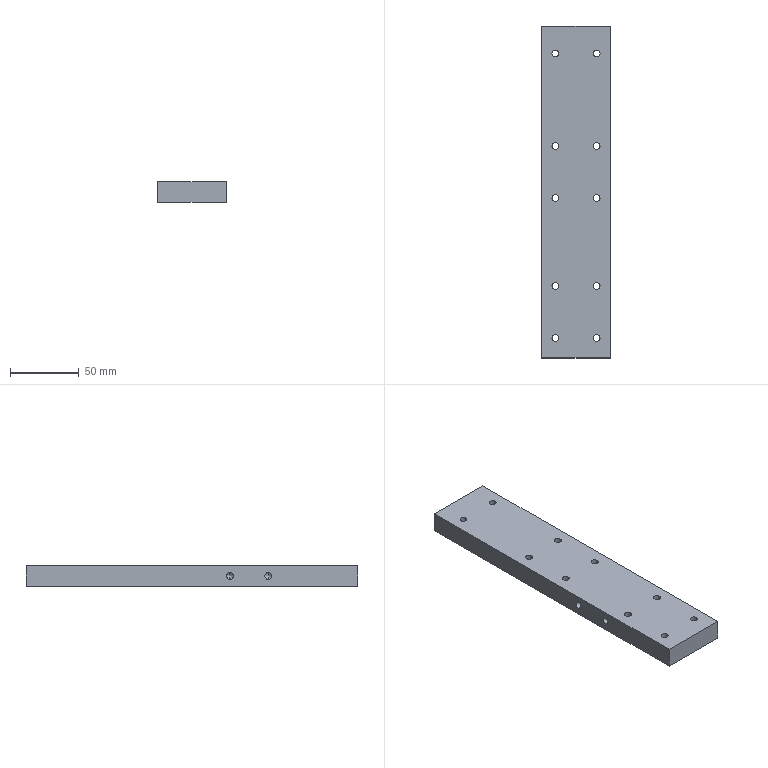Part | 1 solid | 50 faces | box 50 x 242 x 15 mm | volume 176198 mm3 | cylinder 32 | cone 12 | plane 6 | commonest cylinder face diameters 5 x28 6.8 x4
STEP:
#1=CARTESIAN_POINT('',(12.5,124.,15.));
#2=VERTEX_POINT('',#1);
#3=CARTESIAN_POINT('',(17.5,124.,15.));
#4=VERTEX_POINT('',#3);
#5=CARTESIAN_POINT('',(15.,124.,15.));
#6=DIRECTION('',(0.,0.,1.));
#7=DIRECTION('',(1.,0.,0.));
#8=AXIS2_PLACEMENT_3D('',#5,#6,#7);
#9=CIRCLE('',#8,2.5);
#10=EDGE_CURVE('',#2,#4,#9,.T.);
#11=ORIENTED_EDGE('',*,*,#10,.T.);
#12=CARTESIAN_POINT('',(17.5,124.,0.));
#13=VERTEX_POINT('',#12);
#14=CARTESIAN_POINT('',(17.5,124.,0.));
#15=DIRECTION('',(0.,0.,-1.));
#16=VECTOR('',#15,1000.);
#17=LINE('',#14,#16);
#18=EDGE_CURVE('',#4,#13,#17,.T.);
#19=ORIENTED_EDGE('',*,*,#18,.T.);
#20=CARTESIAN_POINT('',(12.5,124.,0.));
#21=VERTEX_POINT('',#20);
#22=CARTESIAN_POINT('',(15.,124.,0.));
#23=DIRECTION('',(0.,0.,-1.));
#24=DIRECTION('',(-1.,0.,0.));
#25=AXIS2_PLACEMENT_3D('',#22,#23,#24);
#26=CIRCLE('',#25,2.5);
#27=EDGE_CURVE('',#13,#21,#26,.T.);
#28=ORIENTED_EDGE('',*,*,#27,.T.);
#29=CARTESIAN_POINT('',(12.5,124.,0.));
#30=DIRECTION('',(0.,0.,-1.));
#31=VECTOR('',#30,1000.);
#32=LINE('',#29,#31);
#33=EDGE_CURVE('',#2,#21,#32,.T.);
#34=ORIENTED_EDGE('',*,*,#33,.F.);
#35=EDGE_LOOP('',(#11,#19,#28,#34));
#36=FACE_OUTER_BOUND('',#35,.T.);
#37=CARTESIAN_POINT('',(15.,124.,0.));
#38=DIRECTION('',(0.,0.,-1.));
#39=DIRECTION('',(-1.,0.,0.));
#40=AXIS2_PLACEMENT_3D('',#37,#38,#39);
#41=CYLINDRICAL_SURFACE('',#40,2.5);
#42=ADVANCED_FACE('',(#36),#41,.F.);
#43=CARTESIAN_POINT('',(-17.5,124.,15.));
#44=VERTEX_POINT('',#43);
#45=CARTESIAN_POINT('',(-12.5,124.,15.));
#46=VERTEX_POINT('',#45);
#47=CARTESIAN_POINT('',(-15.,124.,15.));
#48=DIRECTION('',(0.,0.,1.));
#49=DIRECTION('',(1.,0.,0.));
#50=AXIS2_PLACEMENT_3D('',#47,#48,#49);
#51=CIRCLE('',#50,2.5);
#52=EDGE_CURVE('',#44,#46,#51,.T.);
#53=ORIENTED_EDGE('',*,*,#52,.T.);
#54=CARTESIAN_POINT('',(-12.5,124.,0.));
#55=VERTEX_POINT('',#54);
#56=CARTESIAN_POINT('',(-12.5,124.,0.));
#57=DIRECTION('',(0.,0.,-1.));
#58=VECTOR('',#57,1000.);
#59=LINE('',#56,#58);
#60=EDGE_CURVE('',#46,#55,#59,.T.);
#61=ORIENTED_EDGE('',*,*,#60,.T.);
#62=CARTESIAN_POINT('',(-17.5,124.,0.));
#63=VERTEX_POINT('',#62);
#64=CARTESIAN_POINT('',(-15.,124.,0.));
#65=DIRECTION('',(0.,0.,-1.));
#66=DIRECTION('',(-1.,0.,0.));
#67=AXIS2_PLACEMENT_3D('',#64,#65,#66);
#68=CIRCLE('',#67,2.5);
#69=EDGE_CURVE('',#55,#63,#68,.T.);
#70=ORIENTED_EDGE('',*,*,#69,.T.);
#71=CARTESIAN_POINT('',(-17.5,124.,0.));
#72=DIRECTION('',(0.,0.,-1.));
#73=VECTOR('',#72,1000.);
#74=LINE('',#71,#73);
#75=EDGE_CURVE('',#44,#63,#74,.T.);
#76=ORIENTED_EDGE('',*,*,#75,.F.);
#77=EDGE_LOOP('',(#53,#61,#70,#76));
#78=FACE_OUTER_BOUND('',#77,.T.);
#79=CARTESIAN_POINT('',(-15.,124.,0.));
#80=DIRECTION('',(0.,0.,-1.));
#81=DIRECTION('',(-1.,0.,0.));
#82=AXIS2_PLACEMENT_3D('',#79,#80,#81);
#83=CYLINDRICAL_SURFACE('',#82,2.5);
#84=ADVANCED_FACE('',(#78),#83,.F.);
#85=CARTESIAN_POINT('',(-15.,129.,4.1));
#86=VERTEX_POINT('',#85);
#87=CARTESIAN_POINT('',(-15.,129.,10.9));
#88=VERTEX_POINT('',#87);
#89=CARTESIAN_POINT('',(-15.,129.,7.5));
#90=DIRECTION('',(0.,1.,0.));
#91=DIRECTION('',(0.,0.,1.));
#92=AXIS2_PLACEMENT_3D('',#89,#90,#91);
#93=CIRCLE('',#92,3.4);
#94=EDGE_CURVE('',#86,#88,#93,.T.);
#95=ORIENTED_EDGE('',*,*,#94,.F.);
#96=CARTESIAN_POINT('',(-15.,144.,4.1));
#97=VERTEX_POINT('',#96);
#98=CARTESIAN_POINT('',(-15.,144.,4.1));
#99=DIRECTION('',(0.,1.,0.));
#100=VECTOR('',#99,1000.);
#101=LINE('',#98,#100);
#102=EDGE_CURVE('',#86,#97,#101,.T.);
#103=ORIENTED_EDGE('',*,*,#102,.T.);
#104=CARTESIAN_POINT('',(-15.,144.,10.9));
#105=VERTEX_POINT('',#104);
#106=CARTESIAN_POINT('',(-15.,144.,7.5));
#107=DIRECTION('',(0.,1.,0.));
#108=DIRECTION('',(0.,0.,1.));
#109=AXIS2_PLACEMENT_3D('',#106,#107,#108);
#110=CIRCLE('',#109,3.4);
#111=EDGE_CURVE('',#97,#105,#110,.T.);
#112=ORIENTED_EDGE('',*,*,#111,.T.);
#113=CARTESIAN_POINT('',(-15.,144.,10.9));
#114=DIRECTION('',(0.,1.,0.));
#115=VECTOR('',#114,1000.);
#116=LINE('',#113,#115);
#117=EDGE_CURVE('',#88,#105,#116,.T.);
#118=ORIENTED_EDGE('',*,*,#117,.F.);
#119=EDGE_LOOP('',(#95,#103,#112,#118));
#120=FACE_OUTER_BOUND('',#119,.T.);
#121=CARTESIAN_POINT('',(-15.,144.,7.5));
#122=DIRECTION('',(0.,1.,0.));
#123=DIRECTION('',(0.,0.,1.));
#124=AXIS2_PLACEMENT_3D('',#121,#122,#123);
#125=CYLINDRICAL_SURFACE('',#124,3.4);
#126=ADVANCED_FACE('',(#120),#125,.F.);
#127=CARTESIAN_POINT('',(-15.,126.957,7.5));
#128=VERTEX_POINT('',#127);
#129=CARTESIAN_POINT('',(-15.,129.,10.9));
#130=DIRECTION('',(0.,0.515,0.8572));
#131=VECTOR('',#130,1000.);
#132=LINE('',#129,#131);
#133=EDGE_CURVE('',#128,#88,#132,.T.);
#134=ORIENTED_EDGE('',*,*,#133,.F.);
#135=CARTESIAN_POINT('',(-15.,129.,4.1));
#136=DIRECTION('',(0.,0.515,-0.8572));
#137=VECTOR('',#136,1000.);
#138=LINE('',#135,#137);
#139=EDGE_CURVE('',#128,#86,#138,.T.);
#140=ORIENTED_EDGE('',*,*,#139,.T.);
#141=ORIENTED_EDGE('',*,*,#94,.T.);
#142=EDGE_LOOP('',(#134,#140,#141));
#143=FACE_OUTER_BOUND('',#142,.T.);
#144=CARTESIAN_POINT('',(-15.,129.,7.5));
#145=DIRECTION('',(0.,1.,0.));
#146=DIRECTION('',(0.,0.,1.));
#147=AXIS2_PLACEMENT_3D('',#144,#145,#146);
#148=CONICAL_SURFACE('',#147,3.4,1.03);
#149=ADVANCED_FACE('',(#143),#148,.F.);
#150=CARTESIAN_POINT('',(15.,129.,4.1));
#151=VERTEX_POINT('',#150);
#152=CARTESIAN_POINT('',(15.,129.,10.9));
#153=VERTEX_POINT('',#152);
#154=CARTESIAN_POINT('',(15.,129.,7.5));
#155=DIRECTION('',(0.,1.,0.));
#156=DIRECTION('',(0.,0.,1.));
#157=AXIS2_PLACEMENT_3D('',#154,#155,#156);
#158=CIRCLE('',#157,3.4);
#159=EDGE_CURVE('',#151,#153,#158,.T.);
#160=ORIENTED_EDGE('',*,*,#159,.F.);
#161=CARTESIAN_POINT('',(15.,144.,4.1));
#162=VERTEX_POINT('',#161);
#163=CARTESIAN_POINT('',(15.,144.,4.1));
#164=DIRECTION('',(0.,1.,0.));
#165=VECTOR('',#164,1000.);
#166=LINE('',#163,#165);
#167=EDGE_CURVE('',#151,#162,#166,.T.);
#168=ORIENTED_EDGE('',*,*,#167,.T.);
#169=CARTESIAN_POINT('',(15.,144.,10.9));
#170=VERTEX_POINT('',#169);
#171=CARTESIAN_POINT('',(15.,144.,7.5));
#172=DIRECTION('',(0.,1.,0.));
#173=DIRECTION('',(0.,0.,1.));
#174=AXIS2_PLACEMENT_3D('',#171,#172,#173);
#175=CIRCLE('',#174,3.4);
#176=EDGE_CURVE('',#162,#170,#175,.T.);
#177=ORIENTED_EDGE('',*,*,#176,.T.);
#178=CARTESIAN_POINT('',(15.,144.,10.9));
#179=DIRECTION('',(0.,1.,0.));
#180=VECTOR('',#179,1000.);
#181=LINE('',#178,#180);
#182=EDGE_CURVE('',#153,#170,#181,.T.);
#183=ORIENTED_EDGE('',*,*,#182,.F.);
#184=EDGE_LOOP('',(#160,#168,#177,#183));
#185=FACE_OUTER_BOUND('',#184,.T.);
#186=CARTESIAN_POINT('',(15.,144.,7.5));
#187=DIRECTION('',(0.,1.,0.));
#188=DIRECTION('',(0.,0.,1.));
#189=AXIS2_PLACEMENT_3D('',#186,#187,#188);
#190=CYLINDRICAL_SURFACE('',#189,3.4);
#191=ADVANCED_FACE('',(#185),#190,.F.);
#192=CARTESIAN_POINT('',(15.,126.957,7.5));
#193=VERTEX_POINT('',#192);
#194=CARTESIAN_POINT('',(15.,129.,10.9));
#195=DIRECTION('',(0.,0.515,0.8572));
#196=VECTOR('',#195,1000.);
#197=LINE('',#194,#196);
#198=EDGE_CURVE('',#193,#153,#197,.T.);
#199=ORIENTED_EDGE('',*,*,#198,.F.);
#200=CARTESIAN_POINT('',(15.,129.,4.1));
#201=DIRECTION('',(0.,0.515,-0.8572));
#202=VECTOR('',#201,1000.);
#203=LINE('',#200,#202);
#204=EDGE_CURVE('',#193,#151,#203,.T.);
#205=ORIENTED_EDGE('',*,*,#204,.T.);
#206=ORIENTED_EDGE('',*,*,#159,.T.);
#207=EDGE_LOOP('',(#199,#205,#206));
#208=FACE_OUTER_BOUND('',#207,.T.);
#209=CARTESIAN_POINT('',(15.,129.,7.5));
#210=DIRECTION('',(0.,1.,0.));
#211=DIRECTION('',(0.,0.,1.));
#212=AXIS2_PLACEMENT_3D('',#209,#210,#211);
#213=CONICAL_SURFACE('',#212,3.4,1.03);
#214=ADVANCED_FACE('',(#208),#213,.F.);
#215=CARTESIAN_POINT('',(-10.,-4.64,5.));
#216=VERTEX_POINT('',#215);
#217=CARTESIAN_POINT('',(-10.,-4.64,10.));
#218=VERTEX_POINT('',#217);
#219=CARTESIAN_POINT('',(-10.,-4.64,7.5));
#220=DIRECTION('',(-1.,0.,0.));
#221=DIRECTION('',(0.,0.,1.));
#222=AXIS2_PLACEMENT_3D('',#219,#220,#221);
#223=CIRCLE('',#222,2.5);
#224=EDGE_CURVE('',#216,#218,#223,.T.);
#225=ORIENTED_EDGE('',*,*,#224,.F.);
#226=CARTESIAN_POINT('',(-25.,-4.64,5.));
#227=VERTEX_POINT('',#226);
#228=CARTESIAN_POINT('',(-25.,-4.64,5.));
#229=DIRECTION('',(-1.,0.,0.));
#230=VECTOR('',#229,1000.);
#231=LINE('',#228,#230);
#232=EDGE_CURVE('',#216,#227,#231,.T.);
#233=ORIENTED_EDGE('',*,*,#232,.T.);
#234=CARTESIAN_POINT('',(-25.,-4.64,10.));
#235=VERTEX_POINT('',#234);
#236=CARTESIAN_POINT('',(-25.,-4.64,7.5));
#237=DIRECTION('',(-1.,0.,0.));
#238=DIRECTION('',(0.,0.,1.));
#239=AXIS2_PLACEMENT_3D('',#236,#237,#238);
#240=CIRCLE('',#239,2.5);
#241=EDGE_CURVE('',#227,#235,#240,.T.);
#242=ORIENTED_EDGE('',*,*,#241,.T.);
#243=CARTESIAN_POINT('',(-25.,-4.64,10.));
#244=DIRECTION('',(-1.,0.,0.));
#245=VECTOR('',#244,1000.);
#246=LINE('',#243,#245);
#247=EDGE_CURVE('',#218,#235,#246,.T.);
#248=ORIENTED_EDGE('',*,*,#247,.F.);
#249=EDGE_LOOP('',(#225,#233,#242,#248));
#250=FACE_OUTER_BOUND('',#249,.T.);
#251=CARTESIAN_POINT('',(-25.,-4.64,7.5));
#252=DIRECTION('',(-1.,0.,0.));
#253=DIRECTION('',(0.,0.,1.));
#254=AXIS2_PLACEMENT_3D('',#251,#252,#253);
#255=CYLINDRICAL_SURFACE('',#254,2.5);
#256=ADVANCED_FACE('',(#250),#255,.F.);
#257=CARTESIAN_POINT('',(-8.498,-4.64,7.5));
#258=VERTEX_POINT('',#257);
#259=CARTESIAN_POINT('',(-10.,-4.64,10.));
#260=DIRECTION('',(-0.515,0.,0.8572));
#261=VECTOR('',#260,1000.);
#262=LINE('',#259,#261);
#263=EDGE_CURVE('',#258,#218,#262,.T.);
#264=ORIENTED_EDGE('',*,*,#263,.F.);
#265=CARTESIAN_POINT('',(-10.,-4.64,5.));
#266=DIRECTION('',(-0.515,0.,-0.8572));
#267=VECTOR('',#266,1000.);
#268=LINE('',#265,#267);
#269=EDGE_CURVE('',#258,#216,#268,.T.);
#270=ORIENTED_EDGE('',*,*,#269,.T.);
#271=ORIENTED_EDGE('',*,*,#224,.T.);
#272=EDGE_LOOP('',(#264,#270,#271));
#273=FACE_OUTER_BOUND('',#272,.T.);
#274=CARTESIAN_POINT('',(-10.,-4.64,7.5));
#275=DIRECTION('',(-1.,0.,0.));
#276=DIRECTION('',(0.,0.,1.));
#277=AXIS2_PLACEMENT_3D('',#274,#275,#276);
#278=CONICAL_SURFACE('',#277,2.5,1.03);
#279=ADVANCED_FACE('',(#273),#278,.F.);
#280=CARTESIAN_POINT('',(-10.,-32.64,5.));
#281=VERTEX_POINT('',#280);
#282=CARTESIAN_POINT('',(-10.,-32.64,10.));
#283=VERTEX_POINT('',#282);
#284=CARTESIAN_POINT('',(-10.,-32.64,7.5));
#285=DIRECTION('',(-1.,0.,0.));
#286=DIRECTION('',(0.,0.,1.));
#287=AXIS2_PLACEMENT_3D('',#284,#285,#286);
#288=CIRCLE('',#287,2.5);
#289=EDGE_CURVE('',#281,#283,#288,.T.);
#290=ORIENTED_EDGE('',*,*,#289,.F.);
#291=CARTESIAN_POINT('',(-25.,-32.64,5.));
#292=VERTEX_POINT('',#291);
#293=CARTESIAN_POINT('',(-25.,-32.64,5.));
#294=DIRECTION('',(-1.,0.,0.));
#295=VECTOR('',#294,1000.);
#296=LINE('',#293,#295);
#297=EDGE_CURVE('',#281,#292,#296,.T.);
#298=ORIENTED_EDGE('',*,*,#297,.T.);
#299=CARTESIAN_POINT('',(-25.,-32.64,10.));
#300=VERTEX_POINT('',#299);
#301=CARTESIAN_POINT('',(-25.,-32.64,7.5));
#302=DIRECTION('',(-1.,0.,0.));
#303=DIRECTION('',(0.,0.,1.));
#304=AXIS2_PLACEMENT_3D('',#301,#302,#303);
#305=CIRCLE('',#304,2.5);
#306=EDGE_CURVE('',#292,#300,#305,.T.);
#307=ORIENTED_EDGE('',*,*,#306,.T.);
#308=CARTESIAN_POINT('',(-25.,-32.64,10.));
#309=DIRECTION('',(-1.,0.,0.));
#310=VECTOR('',#309,1000.);
#311=LINE('',#308,#310);
#312=EDGE_CURVE('',#283,#300,#311,.T.);
#313=ORIENTED_EDGE('',*,*,#312,.F.);
#314=EDGE_LOOP('',(#290,#298,#307,#313));
#315=FACE_OUTER_BOUND('',#314,.T.);
#316=CARTESIAN_POINT('',(-25.,-32.64,7.5));
#317=DIRECTION('',(-1.,0.,0.));
#318=DIRECTION('',(0.,0.,1.));
#319=AXIS2_PLACEMENT_3D('',#316,#317,#318);
#320=CYLINDRICAL_SURFACE('',#319,2.5);
#321=ADVANCED_FACE('',(#315),#320,.F.);
#322=CARTESIAN_POINT('',(-8.498,-32.64,7.5));
#323=VERTEX_POINT('',#322);
#324=CARTESIAN_POINT('',(-10.,-32.64,10.));
#325=DIRECTION('',(-0.515,0.,0.8572));
#326=VECTOR('',#325,1000.);
#327=LINE('',#324,#326);
#328=EDGE_CURVE('',#323,#283,#327,.T.);
#329=ORIENTED_EDGE('',*,*,#328,.F.);
#330=CARTESIAN_POINT('',(-10.,-32.64,5.));
#331=DIRECTION('',(-0.515,0.,-0.8572));
#332=VECTOR('',#331,1000.);
#333=LINE('',#330,#332);
#334=EDGE_CURVE('',#323,#281,#333,.T.);
#335=ORIENTED_EDGE('',*,*,#334,.T.);
#336=ORIENTED_EDGE('',*,*,#289,.T.);
#337=EDGE_LOOP('',(#329,#335,#336));
#338=FACE_OUTER_BOUND('',#337,.T.);
#339=CARTESIAN_POINT('',(-10.,-32.64,7.5));
#340=DIRECTION('',(-1.,0.,0.));
#341=DIRECTION('',(0.,0.,1.));
#342=AXIS2_PLACEMENT_3D('',#339,#340,#341);
#343=CONICAL_SURFACE('',#342,2.5,1.03);
#344=ADVANCED_FACE('',(#338),#343,.F.);
#345=CARTESIAN_POINT('',(10.,-4.64,10.));
#346=VERTEX_POINT('',#345);
#347=CARTESIAN_POINT('',(10.,-4.64,5.));
#348=VERTEX_POINT('',#347);
#349=CARTESIAN_POINT('',(10.,-4.64,7.5));
#350=DIRECTION('',(1.,0.,0.));
#351=DIRECTION('',(0.,0.,-1.));
#352=AXIS2_PLACEMENT_3D('',#349,#350,#351);
#353=CIRCLE('',#352,2.5);
#354=EDGE_CURVE('',#346,#348,#353,.T.);
#355=ORIENTED_EDGE('',*,*,#354,.F.);
#356=CARTESIAN_POINT('',(25.,-4.64,10.));
#357=VERTEX_POINT('',#356);
#358=CARTESIAN_POINT('',(25.,-4.64,10.));
#359=DIRECTION('',(1.,0.,0.));
#360=VECTOR('',#359,1000.);
#361=LINE('',#358,#360);
#362=EDGE_CURVE('',#346,#357,#361,.T.);
#363=ORIENTED_EDGE('',*,*,#362,.T.);
#364=CARTESIAN_POINT('',(25.,-4.64,5.));
#365=VERTEX_POINT('',#364);
#366=CARTESIAN_POINT('',(25.,-4.64,7.5));
#367=DIRECTION('',(1.,0.,0.));
#368=DIRECTION('',(0.,0.,-1.));
#369=AXIS2_PLACEMENT_3D('',#366,#367,#368);
#370=CIRCLE('',#369,2.5);
#371=EDGE_CURVE('',#357,#365,#370,.T.);
#372=ORIENTED_EDGE('',*,*,#371,.T.);
#373=CARTESIAN_POINT('',(25.,-4.64,5.));
#374=DIRECTION('',(1.,0.,0.));
#375=VECTOR('',#374,1000.);
#376=LINE('',#373,#375);
#377=EDGE_CURVE('',#348,#365,#376,.T.);
#378=ORIENTED_EDGE('',*,*,#377,.F.);
#379=EDGE_LOOP('',(#355,#363,#372,#378));
#380=FACE_OUTER_BOUND('',#379,.T.);
#381=CARTESIAN_POINT('',(25.,-4.64,7.5));
#382=DIRECTION('',(1.,0.,0.));
#383=DIRECTION('',(0.,0.,-1.));
#384=AXIS2_PLACEMENT_3D('',#381,#382,#383);
#385=CYLINDRICAL_SURFACE('',#384,2.5);
#386=ADVANCED_FACE('',(#380),#385,.F.);
#387=CARTESIAN_POINT('',(8.498,-4.64,7.5));
#388=VERTEX_POINT('',#387);
#389=CARTESIAN_POINT('',(10.,-4.64,5.));
#390=DIRECTION('',(0.515,0.,-0.8572));
#391=VECTOR('',#390,1000.);
#392=LINE('',#389,#391);
#393=EDGE_CURVE('',#388,#348,#392,.T.);
#394=ORIENTED_EDGE('',*,*,#393,.F.);
#395=CARTESIAN_POINT('',(10.,-4.64,10.));
#396=DIRECTION('',(0.515,0.,0.8572));
#397=VECTOR('',#396,1000.);
#398=LINE('',#395,#397);
#399=EDGE_CURVE('',#388,#346,#398,.T.);
#400=ORIENTED_EDGE('',*,*,#399,.T.);
#401=ORIENTED_EDGE('',*,*,#354,.T.);
#402=EDGE_LOOP('',(#394,#400,#401));
#403=FACE_OUTER_BOUND('',#402,.T.);
#404=CARTESIAN_POINT('',(10.,-4.64,7.5));
#405=DIRECTION('',(1.,0.,0.));
#406=DIRECTION('',(0.,0.,-1.));
#407=AXIS2_PLACEMENT_3D('',#404,#405,#406);
#408=CONICAL_SURFACE('',#407,2.5,1.03);
#409=ADVANCED_FACE('',(#403),#408,.F.);
#410=CARTESIAN_POINT('',(10.,-32.64,10.));
#411=VERTEX_POINT('',#410);
#412=CARTESIAN_POINT('',(10.,-32.64,5.));
#413=VERTEX_POINT('',#412);
#414=CARTESIAN_POINT('',(10.,-32.64,7.5));
#415=DIRECTION('',(1.,0.,0.));
#416=DIRECTION('',(0.,0.,-1.));
#417=AXIS2_PLACEMENT_3D('',#414,#415,#416);
#418=CIRCLE('',#417,2.5);
#419=EDGE_CURVE('',#411,#413,#418,.T.);
#420=ORIENTED_EDGE('',*,*,#419,.F.);
#421=CARTESIAN_POINT('',(25.,-32.64,10.));
#422=VERTEX_POINT('',#421);
#423=CARTESIAN_POINT('',(25.,-32.64,10.));
#424=DIRECTION('',(1.,0.,0.));
#425=VECTOR('',#424,1000.);
#426=LINE('',#423,#425);
#427=EDGE_CURVE('',#411,#422,#426,.T.);
#428=ORIENTED_EDGE('',*,*,#427,.T.);
#429=CARTESIAN_POINT('',(25.,-32.64,5.));
#430=VERTEX_POINT('',#429);
#431=CARTESIAN_POINT('',(25.,-32.64,7.5));
#432=DIRECTION('',(1.,0.,0.));
#433=DIRECTION('',(0.,0.,-1.));
#434=AXIS2_PLACEMENT_3D('',#431,#432,#433);
#435=CIRCLE('',#434,2.5);
#436=EDGE_CURVE('',#422,#430,#435,.T.);
#437=ORIENTED_EDGE('',*,*,#436,.T.);
#438=CARTESIAN_POINT('',(25.,-32.64,5.));
#439=DIRECTION('',(1.,0.,0.));
#440=VECTOR('',#439,1000.);
#441=LINE('',#438,#440);
#442=EDGE_CURVE('',#413,#430,#441,.T.);
#443=ORIENTED_EDGE('',*,*,#442,.F.);
#444=EDGE_LOOP('',(#420,#428,#437,#443));
#445=FACE_OUTER_BOUND('',#444,.T.);
#446=CARTESIAN_POINT('',(25.,-32.64,7.5));
#447=DIRECTION('',(1.,0.,0.));
#448=DIRECTION('',(0.,0.,-1.));
#449=AXIS2_PLACEMENT_3D('',#446,#447,#448);
#450=CYLINDRICAL_SURFACE('',#449,2.5);
#451=ADVANCED_FACE('',(#445),#450,.F.);
#452=CARTESIAN_POINT('',(8.498,-32.64,7.5));
#453=VERTEX_POINT('',#452);
#454=CARTESIAN_POINT('',(10.,-32.64,5.));
#455=DIRECTION('',(0.515,0.,-0.8572));
#456=VECTOR('',#455,1000.);
#457=LINE('',#454,#456);
#458=EDGE_CURVE('',#453,#413,#457,.T.);
#459=ORIENTED_EDGE('',*,*,#458,.F.);
#460=CARTESIAN_POINT('',(10.,-32.64,10.));
#461=DIRECTION('',(0.515,0.,0.8572));
#462=VECTOR('',#461,1000.);
#463=LINE('',#460,#462);
#464=EDGE_CURVE('',#453,#411,#463,.T.);
#465=ORIENTED_EDGE('',*,*,#464,.T.);
#466=ORIENTED_EDGE('',*,*,#419,.T.);
#467=EDGE_LOOP('',(#459,#465,#466));
#468=FACE_OUTER_BOUND('',#467,.T.);
#469=CARTESIAN_POINT('',(10.,-32.64,7.5));
#470=DIRECTION('',(1.,0.,0.));
#471=DIRECTION('',(0.,0.,-1.));
#472=AXIS2_PLACEMENT_3D('',#469,#470,#471);
#473=CONICAL_SURFACE('',#472,2.5,1.03);
#474=ADVANCED_FACE('',(#468),#473,.F.);
#475=CARTESIAN_POINT('',(-17.5,-83.5,15.));
#476=VERTEX_POINT('',#475);
#477=CARTESIAN_POINT('',(-12.5,-83.5,15.));
#478=VERTEX_POINT('',#477);
#479=CARTESIAN_POINT('',(-15.,-83.5,15.));
#480=DIRECTION('',(0.,0.,1.));
#481=DIRECTION('',(1.,0.,0.));
#482=AXIS2_PLACEMENT_3D('',#479,#480,#481);
#483=CIRCLE('',#482,2.5);
#484=EDGE_CURVE('',#476,#478,#483,.T.);
#485=ORIENTED_EDGE('',*,*,#484,.T.);
#486=CARTESIAN_POINT('',(-12.5,-83.5,0.));
#487=VERTEX_POINT('',#486);
#488=CARTESIAN_POINT('',(-12.5,-83.5,38.));
#489=DIRECTION('',(0.,0.,-1.));
#490=VECTOR('',#489,1000.);
#491=LINE('',#488,#490);
#492=EDGE_CURVE('',#478,#487,#491,.T.);
#493=ORIENTED_EDGE('',*,*,#492,.T.);
#494=CARTESIAN_POINT('',(-17.5,-83.5,0.));
#495=VERTEX_POINT('',#494);
#496=CARTESIAN_POINT('',(-15.,-83.5,0.));
#497=DIRECTION('',(0.,0.,-1.));
#498=DIRECTION('',(-1.,0.,0.));
#499=AXIS2_PLACEMENT_3D('',#496,#497,#498);
#500=CIRCLE('',#499,2.5);
#501=EDGE_CURVE('',#487,#495,#500,.T.);
#502=ORIENTED_EDGE('',*,*,#501,.T.);
#503=CARTESIAN_POINT('',(-17.5,-83.5,38.));
#504=DIRECTION('',(0.,0.,-1.));
#505=VECTOR('',#504,1000.);
#506=LINE('',#503,#505);
#507=EDGE_CURVE('',#476,#495,#506,.T.);
#508=ORIENTED_EDGE('',*,*,#507,.F.);
#509=EDGE_LOOP('',(#485,#493,#502,#508));
#510=FACE_OUTER_BOUND('',#509,.T.);
#511=CARTESIAN_POINT('',(-15.,-83.5,38.));
#512=DIRECTION('',(0.,0.,-1.));
#513=DIRECTION('',(-1.,0.,0.));
#514=AXIS2_PLACEMENT_3D('',#511,#512,#513);
#515=CYLINDRICAL_SURFACE('',#514,2.5);
#516=ADVANCED_FACE('',(#510),#515,.F.);
#517=CARTESIAN_POINT('',(12.5,-83.5,15.));
#518=VERTEX_POINT('',#517);
#519=CARTESIAN_POINT('',(17.5,-83.5,15.));
#520=VERTEX_POINT('',#519);
#521=CARTESIAN_POINT('',(15.,-83.5,15.));
#522=DIRECTION('',(0.,0.,1.));
#523=DIRECTION('',(1.,0.,0.));
#524=AXIS2_PLACEMENT_3D('',#521,#522,#523);
#525=CIRCLE('',#524,2.5);
#526=EDGE_CURVE('',#518,#520,#525,.T.);
#527=ORIENTED_EDGE('',*,*,#526,.T.);
#528=CARTESIAN_POINT('',(17.5,-83.5,0.));
#529=VERTEX_POINT('',#528);
#530=CARTESIAN_POINT('',(17.5,-83.5,38.));
#531=DIRECTION('',(0.,0.,-1.));
#532=VECTOR('',#531,1000.);
#533=LINE('',#530,#532);
#534=EDGE_CURVE('',#520,#529,#533,.T.);
#535=ORIENTED_EDGE('',*,*,#534,.T.);
#536=CARTESIAN_POINT('',(12.5,-83.5,0.));
#537=VERTEX_POINT('',#536);
#538=CARTESIAN_POINT('',(15.,-83.5,0.));
#539=DIRECTION('',(0.,0.,-1.));
#540=DIRECTION('',(-1.,0.,0.));
#541=AXIS2_PLACEMENT_3D('',#538,#539,#540);
#542=CIRCLE('',#541,2.5);
#543=EDGE_CURVE('',#529,#537,#542,.T.);
#544=ORIENTED_EDGE('',*,*,#543,.T.);
#545=CARTESIAN_POINT('',(12.5,-83.5,38.));
#546=DIRECTION('',(0.,0.,-1.));
#547=VECTOR('',#546,1000.);
#548=LINE('',#545,#547);
#549=EDGE_CURVE('',#518,#537,#548,.T.);
#550=ORIENTED_EDGE('',*,*,#549,.F.);
#551=EDGE_LOOP('',(#527,#535,#544,#550));
#552=FACE_OUTER_BOUND('',#551,.T.);
#553=CARTESIAN_POINT('',(15.,-83.5,38.));
#554=DIRECTION('',(0.,0.,-1.));
#555=DIRECTION('',(-1.,0.,0.));
#556=AXIS2_PLACEMENT_3D('',#553,#554,#555);
#557=CYLINDRICAL_SURFACE('',#556,2.5);
#558=ADVANCED_FACE('',(#552),#557,.F.);
#559=CARTESIAN_POINT('',(-17.5,-45.5,15.));
#560=VERTEX_POINT('',#559);
#561=CARTESIAN_POINT('',(-12.5,-45.5,15.));
#562=VERTEX_POINT('',#561);
#563=CARTESIAN_POINT('',(-15.,-45.5,15.));
#564=DIRECTION('',(0.,0.,1.));
#565=DIRECTION('',(1.,0.,0.));
#566=AXIS2_PLACEMENT_3D('',#563,#564,#565);
#567=CIRCLE('',#566,2.5);
#568=EDGE_CURVE('',#560,#562,#567,.T.);
#569=ORIENTED_EDGE('',*,*,#568,.T.);
#570=CARTESIAN_POINT('',(-12.5,-45.5,0.));
#571=VERTEX_POINT('',#570);
#572=CARTESIAN_POINT('',(-12.5,-45.5,38.));
#573=DIRECTION('',(0.,0.,-1.));
#574=VECTOR('',#573,1000.);
#575=LINE('',#572,#574);
#576=EDGE_CURVE('',#562,#571,#575,.T.);
#577=ORIENTED_EDGE('',*,*,#576,.T.);
#578=CARTESIAN_POINT('',(-17.5,-45.5,0.));
#579=VERTEX_POINT('',#578);
#580=CARTESIAN_POINT('',(-15.,-45.5,0.));
#581=DIRECTION('',(0.,0.,-1.));
#582=DIRECTION('',(-1.,0.,0.));
#583=AXIS2_PLACEMENT_3D('',#580,#581,#582);
#584=CIRCLE('',#583,2.5);
#585=EDGE_CURVE('',#571,#579,#584,.T.);
#586=ORIENTED_EDGE('',*,*,#585,.T.);
#587=CARTESIAN_POINT('',(-17.5,-45.5,38.));
#588=DIRECTION('',(0.,0.,-1.));
#589=VECTOR('',#588,1000.);
#590=LINE('',#587,#589);
#591=EDGE_CURVE('',#560,#579,#590,.T.);
#592=ORIENTED_EDGE('',*,*,#591,.F.);
#593=EDGE_LOOP('',(#569,#577,#586,#592));
#594=FACE_OUTER_BOUND('',#593,.T.);
#595=CARTESIAN_POINT('',(-15.,-45.5,38.));
#596=DIRECTION('',(0.,0.,-1.));
#597=DIRECTION('',(-1.,0.,0.));
#598=AXIS2_PLACEMENT_3D('',#595,#596,#597);
#599=CYLINDRICAL_SURFACE('',#598,2.5);
#600=ADVANCED_FACE('',(#594),#599,.F.);
#601=CARTESIAN_POINT('',(12.5,-45.5,15.));
#602=VERTEX_POINT('',#601);
#603=CARTESIAN_POINT('',(17.5,-45.5,15.));
#604=VERTEX_POINT('',#603);
#605=CARTESIAN_POINT('',(15.,-45.5,15.));
#606=DIRECTION('',(0.,0.,1.));
#607=DIRECTION('',(1.,0.,0.));
#608=AXIS2_PLACEMENT_3D('',#605,#606,#607);
#609=CIRCLE('',#608,2.5);
#610=EDGE_CURVE('',#602,#604,#609,.T.);
#611=ORIENTED_EDGE('',*,*,#610,.T.);
#612=CARTESIAN_POINT('',(17.5,-45.5,0.));
#613=VERTEX_POINT('',#612);
#614=CARTESIAN_POINT('',(17.5,-45.5,38.));
#615=DIRECTION('',(0.,0.,-1.));
#616=VECTOR('',#615,1000.);
#617=LINE('',#614,#616);
#618=EDGE_CURVE('',#604,#613,#617,.T.);
#619=ORIENTED_EDGE('',*,*,#618,.T.);
#620=CARTESIAN_POINT('',(12.5,-45.5,0.));
#621=VERTEX_POINT('',#620);
#622=CARTESIAN_POINT('',(15.,-45.5,0.));
#623=DIRECTION('',(0.,0.,-1.));
#624=DIRECTION('',(-1.,0.,0.));
#625=AXIS2_PLACEMENT_3D('',#622,#623,#624);
#626=CIRCLE('',#625,2.5);
#627=EDGE_CURVE('',#613,#621,#626,.T.);
#628=ORIENTED_EDGE('',*,*,#627,.T.);
#629=CARTESIAN_POINT('',(12.5,-45.5,38.));
#630=DIRECTION('',(0.,0.,-1.));
#631=VECTOR('',#630,1000.);
#632=LINE('',#629,#631);
#633=EDGE_CURVE('',#602,#621,#632,.T.);
#634=ORIENTED_EDGE('',*,*,#633,.F.);
#635=EDGE_LOOP('',(#611,#619,#628,#634));
#636=FACE_OUTER_BOUND('',#635,.T.);
#637=CARTESIAN_POINT('',(15.,-45.5,38.));
#638=DIRECTION('',(0.,0.,-1.));
#639=DIRECTION('',(-1.,0.,0.));
#640=AXIS2_PLACEMENT_3D('',#637,#638,#639);
#641=CYLINDRICAL_SURFACE('',#640,2.5);
#642=ADVANCED_FACE('',(#636),#641,.F.);
#643=CARTESIAN_POINT('',(-17.5,18.5,15.));
#644=VERTEX_POINT('',#643);
#645=CARTESIAN_POINT('',(-12.5,18.5,15.));
#646=VERTEX_POINT('',#645);
#647=CARTESIAN_POINT('',(-15.,18.5,15.));
#648=DIRECTION('',(0.,0.,1.));
#649=DIRECTION('',(1.,0.,0.));
#650=AXIS2_PLACEMENT_3D('',#647,#648,#649);
#651=CIRCLE('',#650,2.5);
#652=EDGE_CURVE('',#644,#646,#651,.T.);
#653=ORIENTED_EDGE('',*,*,#652,.T.);
#654=CARTESIAN_POINT('',(-12.5,18.5,0.));
#655=VERTEX_POINT('',#654);
#656=CARTESIAN_POINT('',(-12.5,18.5,38.));
#657=DIRECTION('',(0.,0.,-1.));
#658=VECTOR('',#657,1000.);
#659=LINE('',#656,#658);
#660=EDGE_CURVE('',#646,#655,#659,.T.);
#661=ORIENTED_EDGE('',*,*,#660,.T.);
#662=CARTESIAN_POINT('',(-17.5,18.5,0.));
#663=VERTEX_POINT('',#662);
#664=CARTESIAN_POINT('',(-15.,18.5,0.));
#665=DIRECTION('',(0.,0.,-1.));
#666=DIRECTION('',(-1.,0.,0.));
#667=AXIS2_PLACEMENT_3D('',#664,#665,#666);
#668=CIRCLE('',#667,2.5);
#669=EDGE_CURVE('',#655,#663,#668,.T.);
#670=ORIENTED_EDGE('',*,*,#669,.T.);
#671=CARTESIAN_POINT('',(-17.5,18.5,38.));
#672=DIRECTION('',(0.,0.,-1.));
#673=VECTOR('',#672,1000.);
#674=LINE('',#671,#673);
#675=EDGE_CURVE('',#644,#663,#674,.T.);
#676=ORIENTED_EDGE('',*,*,#675,.F.);
#677=EDGE_LOOP('',(#653,#661,#670,#676));
#678=FACE_OUTER_BOUND('',#677,.T.);
#679=CARTESIAN_POINT('',(-15.,18.5,38.));
#680=DIRECTION('',(0.,0.,-1.));
#681=DIRECTION('',(-1.,0.,0.));
#682=AXIS2_PLACEMENT_3D('',#679,#680,#681);
#683=CYLINDRICAL_SURFACE('',#682,2.5);
#684=ADVANCED_FACE('',(#678),#683,.F.);
#685=CARTESIAN_POINT('',(12.5,18.5,15.));
#686=VERTEX_POINT('',#685);
#687=CARTESIAN_POINT('',(17.5,18.5,15.));
#688=VERTEX_POINT('',#687);
#689=CARTESIAN_POINT('',(15.,18.5,15.));
#690=DIRECTION('',(0.,0.,1.));
#691=DIRECTION('',(1.,0.,0.));
#692=AXIS2_PLACEMENT_3D('',#689,#690,#691);
#693=CIRCLE('',#692,2.5);
#694=EDGE_CURVE('',#686,#688,#693,.T.);
#695=ORIENTED_EDGE('',*,*,#694,.T.);
#696=CARTESIAN_POINT('',(17.5,18.5,0.));
#697=VERTEX_POINT('',#696);
#698=CARTESIAN_POINT('',(17.5,18.5,38.));
#699=DIRECTION('',(0.,0.,-1.));
#700=VECTOR('',#699,1000.);
#701=LINE('',#698,#700);
#702=EDGE_CURVE('',#688,#697,#701,.T.);
#703=ORIENTED_EDGE('',*,*,#702,.T.);
#704=CARTESIAN_POINT('',(12.5,18.5,0.));
#705=VERTEX_POINT('',#704);
#706=CARTESIAN_POINT('',(15.,18.5,0.));
#707=DIRECTION('',(0.,0.,-1.));
#708=DIRECTION('',(-1.,0.,0.));
#709=AXIS2_PLACEMENT_3D('',#706,#707,#708);
#710=CIRCLE('',#709,2.5);
#711=EDGE_CURVE('',#697,#705,#710,.T.);
#712=ORIENTED_EDGE('',*,*,#711,.T.);
#713=CARTESIAN_POINT('',(12.5,18.5,38.));
#714=DIRECTION('',(0.,0.,-1.));
#715=VECTOR('',#714,1000.);
#716=LINE('',#713,#715);
#717=EDGE_CURVE('',#686,#705,#716,.T.);
#718=ORIENTED_EDGE('',*,*,#717,.F.);
#719=EDGE_LOOP('',(#695,#703,#712,#718));
#720=FACE_OUTER_BOUND('',#719,.T.);
#721=CARTESIAN_POINT('',(15.,18.5,38.));
#722=DIRECTION('',(0.,0.,-1.));
#723=DIRECTION('',(-1.,0.,0.));
#724=AXIS2_PLACEMENT_3D('',#721,#722,#723);
#725=CYLINDRICAL_SURFACE('',#724,2.5);
#726=ADVANCED_FACE('',(#720),#725,.F.);
#727=CARTESIAN_POINT('',(-17.5,56.5,15.));
#728=VERTEX_POINT('',#727);
#729=CARTESIAN_POINT('',(-12.5,56.5,15.));
#730=VERTEX_POINT('',#729);
#731=CARTESIAN_POINT('',(-15.,56.5,15.));
#732=DIRECTION('',(0.,0.,1.));
#733=DIRECTION('',(1.,0.,0.));
#734=AXIS2_PLACEMENT_3D('',#731,#732,#733);
#735=CIRCLE('',#734,2.5);
#736=EDGE_CURVE('',#728,#730,#735,.T.);
#737=ORIENTED_EDGE('',*,*,#736,.T.);
#738=CARTESIAN_POINT('',(-12.5,56.5,0.));
#739=VERTEX_POINT('',#738);
#740=CARTESIAN_POINT('',(-12.5,56.5,38.));
#741=DIRECTION('',(0.,0.,-1.));
#742=VECTOR('',#741,1000.);
#743=LINE('',#740,#742);
#744=EDGE_CURVE('',#730,#739,#743,.T.);
#745=ORIENTED_EDGE('',*,*,#744,.T.);
#746=CARTESIAN_POINT('',(-17.5,56.5,0.));
#747=VERTEX_POINT('',#746);
#748=CARTESIAN_POINT('',(-15.,56.5,0.));
#749=DIRECTION('',(0.,0.,-1.));
#750=DIRECTION('',(-1.,0.,0.));
#751=AXIS2_PLACEMENT_3D('',#748,#749,#750);
#752=CIRCLE('',#751,2.5);
#753=EDGE_CURVE('',#739,#747,#752,.T.);
#754=ORIENTED_EDGE('',*,*,#753,.T.);
#755=CARTESIAN_POINT('',(-17.5,56.5,38.));
#756=DIRECTION('',(0.,0.,-1.));
#757=VECTOR('',#756,1000.);
#758=LINE('',#755,#757);
#759=EDGE_CURVE('',#728,#747,#758,.T.);
#760=ORIENTED_EDGE('',*,*,#759,.F.);
#761=EDGE_LOOP('',(#737,#745,#754,#760));
#762=FACE_OUTER_BOUND('',#761,.T.);
#763=CARTESIAN_POINT('',(-15.,56.5,38.));
#764=DIRECTION('',(0.,0.,-1.));
#765=DIRECTION('',(-1.,0.,0.));
#766=AXIS2_PLACEMENT_3D('',#763,#764,#765);
#767=CYLINDRICAL_SURFACE('',#766,2.5);
#768=ADVANCED_FACE('',(#762),#767,.F.);
#769=CARTESIAN_POINT('',(12.5,56.5,15.));
#770=VERTEX_POINT('',#769);
#771=CARTESIAN_POINT('',(17.5,56.5,15.));
#772=VERTEX_POINT('',#771);
#773=CARTESIAN_POINT('',(15.,56.5,15.));
#774=DIRECTION('',(0.,0.,1.));
#775=DIRECTION('',(1.,0.,0.));
#776=AXIS2_PLACEMENT_3D('',#773,#774,#775);
#777=CIRCLE('',#776,2.5);
#778=EDGE_CURVE('',#770,#772,#777,.T.);
#779=ORIENTED_EDGE('',*,*,#778,.T.);
#780=CARTESIAN_POINT('',(17.5,56.5,0.));
#781=VERTEX_POINT('',#780);
#782=CARTESIAN_POINT('',(17.5,56.5,38.));
#783=DIRECTION('',(0.,0.,-1.));
#784=VECTOR('',#783,1000.);
#785=LINE('',#782,#784);
#786=EDGE_CURVE('',#772,#781,#785,.T.);
#787=ORIENTED_EDGE('',*,*,#786,.T.);
#788=CARTESIAN_POINT('',(12.5,56.5,0.));
#789=VERTEX_POINT('',#788);
#790=CARTESIAN_POINT('',(15.,56.5,0.));
#791=DIRECTION('',(0.,0.,-1.));
#792=DIRECTION('',(-1.,0.,0.));
#793=AXIS2_PLACEMENT_3D('',#790,#791,#792);
#794=CIRCLE('',#793,2.5);
#795=EDGE_CURVE('',#781,#789,#794,.T.);
#796=ORIENTED_EDGE('',*,*,#795,.T.);
#797=CARTESIAN_POINT('',(12.5,56.5,38.));
#798=DIRECTION('',(0.,0.,-1.));
#799=VECTOR('',#798,1000.);
#800=LINE('',#797,#799);
#801=EDGE_CURVE('',#770,#789,#800,.T.);
#802=ORIENTED_EDGE('',*,*,#801,.F.);
#803=EDGE_LOOP('',(#779,#787,#796,#802));
#804=FACE_OUTER_BOUND('',#803,.T.);
#805=CARTESIAN_POINT('',(15.,56.5,38.));
#806=DIRECTION('',(0.,0.,-1.));
#807=DIRECTION('',(-1.,0.,0.));
#808=AXIS2_PLACEMENT_3D('',#805,#806,#807);
#809=CYLINDRICAL_SURFACE('',#808,2.5);
#810=ADVANCED_FACE('',(#804),#809,.F.);
#811=CARTESIAN_POINT('',(25.,-4.64,7.5));
#812=DIRECTION('',(1.,0.,0.));
#813=DIRECTION('',(0.,0.,-1.));
#814=AXIS2_PLACEMENT_3D('',#811,#812,#813);
#815=CIRCLE('',#814,2.5);
#816=EDGE_CURVE('',#365,#357,#815,.T.);
#817=ORIENTED_EDGE('',*,*,#816,.F.);
#818=ORIENTED_EDGE('',*,*,#371,.F.);
#819=EDGE_LOOP('',(#817,#818));
#820=FACE_BOUND('',#819,.T.);
#821=CARTESIAN_POINT('',(25.,-98.,0.));
#822=VERTEX_POINT('',#821);
#823=CARTESIAN_POINT('',(25.,-98.,15.));
#824=VERTEX_POINT('',#823);
#825=CARTESIAN_POINT('',(25.,-98.,0.));
#826=DIRECTION('',(0.,0.,1.));
#827=VECTOR('',#826,1000.);
#828=LINE('',#825,#827);
#829=EDGE_CURVE('',#822,#824,#828,.T.);
#830=ORIENTED_EDGE('',*,*,#829,.F.);
#831=CARTESIAN_POINT('',(25.,144.,0.));
#832=VERTEX_POINT('',#831);
#833=CARTESIAN_POINT('',(25.,-119.,0.));
#834=DIRECTION('',(0.,1.,0.));
#835=VECTOR('',#834,1000.);
#836=LINE('',#833,#835);
#837=EDGE_CURVE('',#822,#832,#836,.T.);
#838=ORIENTED_EDGE('',*,*,#837,.T.);
#839=CARTESIAN_POINT('',(25.,144.,15.));
#840=VERTEX_POINT('',#839);
#841=CARTESIAN_POINT('',(25.,144.,15.));
#842=DIRECTION('',(0.,0.,-1.));
#843=VECTOR('',#842,1000.);
#844=LINE('',#841,#843);
#845=EDGE_CURVE('',#840,#832,#844,.T.);
#846=ORIENTED_EDGE('',*,*,#845,.F.);
#847=CARTESIAN_POINT('',(25.,-119.,15.));
#848=DIRECTION('',(0.,1.,0.));
#849=VECTOR('',#848,1000.);
#850=LINE('',#847,#849);
#851=EDGE_CURVE('',#824,#840,#850,.T.);
#852=ORIENTED_EDGE('',*,*,#851,.F.);
#853=EDGE_LOOP('',(#830,#838,#846,#852));
#854=FACE_OUTER_BOUND('',#853,.T.);
#855=CARTESIAN_POINT('',(25.,-32.64,7.5));
#856=DIRECTION('',(1.,0.,0.));
#857=DIRECTION('',(0.,0.,-1.));
#858=AXIS2_PLACEMENT_3D('',#855,#856,#857);
#859=CIRCLE('',#858,2.5);
#860=EDGE_CURVE('',#430,#422,#859,.T.);
#861=ORIENTED_EDGE('',*,*,#860,.F.);
#862=ORIENTED_EDGE('',*,*,#436,.F.);
#863=EDGE_LOOP('',(#861,#862));
#864=FACE_BOUND('',#863,.T.);
#865=CARTESIAN_POINT('',(25.,-119.,15.));
#866=DIRECTION('',(-1.,0.,0.));
#867=DIRECTION('',(0.,0.,1.));
#868=AXIS2_PLACEMENT_3D('',#865,#866,#867);
#869=PLANE('',#868);
#870=ADVANCED_FACE('',(#820,#854,#864),#869,.F.);
#871=CARTESIAN_POINT('',(-25.,-4.64,7.5));
#872=DIRECTION('',(-1.,0.,0.));
#873=DIRECTION('',(0.,0.,1.));
#874=AXIS2_PLACEMENT_3D('',#871,#872,#873);
#875=CIRCLE('',#874,2.5);
#876=EDGE_CURVE('',#235,#227,#875,.T.);
#877=ORIENTED_EDGE('',*,*,#876,.F.);
#878=ORIENTED_EDGE('',*,*,#241,.F.);
#879=EDGE_LOOP('',(#877,#878));
#880=FACE_BOUND('',#879,.T.);
#881=CARTESIAN_POINT('',(-25.,-32.64,7.5));
#882=DIRECTION('',(-1.,0.,0.));
#883=DIRECTION('',(0.,0.,1.));
#884=AXIS2_PLACEMENT_3D('',#881,#882,#883);
#885=CIRCLE('',#884,2.5);
#886=EDGE_CURVE('',#300,#292,#885,.T.);
#887=ORIENTED_EDGE('',*,*,#886,.F.);
#888=ORIENTED_EDGE('',*,*,#306,.F.);
#889=EDGE_LOOP('',(#887,#888));
#890=FACE_BOUND('',#889,.T.);
#891=CARTESIAN_POINT('',(-25.,-98.,15.));
#892=VERTEX_POINT('',#891);
#893=CARTESIAN_POINT('',(-25.,-98.,0.));
#894=VERTEX_POINT('',#893);
#895=CARTESIAN_POINT('',(-25.,-98.,15.));
#896=DIRECTION('',(0.,0.,-1.));
#897=VECTOR('',#896,1000.);
#898=LINE('',#895,#897);
#899=EDGE_CURVE('',#892,#894,#898,.T.);
#900=ORIENTED_EDGE('',*,*,#899,.F.);
#901=CARTESIAN_POINT('',(-25.,144.,15.));
#902=VERTEX_POINT('',#901);
#903=CARTESIAN_POINT('',(-25.,-119.,15.));
#904=DIRECTION('',(0.,-1.,0.));
#905=VECTOR('',#904,1000.);
#906=LINE('',#903,#905);
#907=EDGE_CURVE('',#902,#892,#906,.T.);
#908=ORIENTED_EDGE('',*,*,#907,.F.);
#909=CARTESIAN_POINT('',(-25.,144.,0.));
#910=VERTEX_POINT('',#909);
#911=CARTESIAN_POINT('',(-25.,144.,0.));
#912=DIRECTION('',(0.,0.,1.));
#913=VECTOR('',#912,1000.);
#914=LINE('',#911,#913);
#915=EDGE_CURVE('',#910,#902,#914,.T.);
#916=ORIENTED_EDGE('',*,*,#915,.F.);
#917=CARTESIAN_POINT('',(-25.,-119.,0.));
#918=DIRECTION('',(0.,-1.,0.));
#919=VECTOR('',#918,1000.);
#920=LINE('',#917,#919);
#921=EDGE_CURVE('',#910,#894,#920,.T.);
#922=ORIENTED_EDGE('',*,*,#921,.T.);
#923=EDGE_LOOP('',(#900,#908,#916,#922));
#924=FACE_OUTER_BOUND('',#923,.T.);
#925=CARTESIAN_POINT('',(-25.,-119.,15.));
#926=DIRECTION('',(1.,0.,0.));
#927=DIRECTION('',(0.,0.,-1.));
#928=AXIS2_PLACEMENT_3D('',#925,#926,#927);
#929=PLANE('',#928);
#930=ADVANCED_FACE('',(#880,#890,#924),#929,.F.);
#931=ORIENTED_EDGE('',*,*,#10,.F.);
#932=CARTESIAN_POINT('',(15.,124.,15.));
#933=DIRECTION('',(0.,0.,1.));
#934=DIRECTION('',(1.,0.,0.));
#935=AXIS2_PLACEMENT_3D('',#932,#933,#934);
#936=CIRCLE('',#935,2.5);
#937=EDGE_CURVE('',#4,#2,#936,.T.);
#938=ORIENTED_EDGE('',*,*,#937,.F.);
#939=EDGE_LOOP('',(#931,#938));
#940=FACE_BOUND('',#939,.T.);
#941=ORIENTED_EDGE('',*,*,#52,.F.);
#942=CARTESIAN_POINT('',(-15.,124.,15.));
#943=DIRECTION('',(0.,0.,1.));
#944=DIRECTION('',(1.,0.,0.));
#945=AXIS2_PLACEMENT_3D('',#942,#943,#944);
#946=CIRCLE('',#945,2.5);
#947=EDGE_CURVE('',#46,#44,#946,.T.);
#948=ORIENTED_EDGE('',*,*,#947,.F.);
#949=EDGE_LOOP('',(#941,#948));
#950=FACE_BOUND('',#949,.T.);
#951=ORIENTED_EDGE('',*,*,#484,.F.);
#952=CARTESIAN_POINT('',(-15.,-83.5,15.));
#953=DIRECTION('',(0.,0.,1.));
#954=DIRECTION('',(1.,0.,0.));
#955=AXIS2_PLACEMENT_3D('',#952,#953,#954);
#956=CIRCLE('',#955,2.5);
#957=EDGE_CURVE('',#478,#476,#956,.T.);
#958=ORIENTED_EDGE('',*,*,#957,.F.);
#959=EDGE_LOOP('',(#951,#958));
#960=FACE_BOUND('',#959,.T.);
#961=ORIENTED_EDGE('',*,*,#526,.F.);
#962=CARTESIAN_POINT('',(15.,-83.5,15.));
#963=DIRECTION('',(0.,0.,1.));
#964=DIRECTION('',(1.,0.,0.));
#965=AXIS2_PLACEMENT_3D('',#962,#963,#964);
#966=CIRCLE('',#965,2.5);
#967=EDGE_CURVE('',#520,#518,#966,.T.);
#968=ORIENTED_EDGE('',*,*,#967,.F.);
#969=EDGE_LOOP('',(#961,#968));
#970=FACE_BOUND('',#969,.T.);
#971=ORIENTED_EDGE('',*,*,#568,.F.);
#972=CARTESIAN_POINT('',(-15.,-45.5,15.));
#973=DIRECTION('',(0.,0.,1.));
#974=DIRECTION('',(1.,0.,0.));
#975=AXIS2_PLACEMENT_3D('',#972,#973,#974);
#976=CIRCLE('',#975,2.5);
#977=EDGE_CURVE('',#562,#560,#976,.T.);
#978=ORIENTED_EDGE('',*,*,#977,.F.);
#979=EDGE_LOOP('',(#971,#978));
#980=FACE_BOUND('',#979,.T.);
#981=ORIENTED_EDGE('',*,*,#610,.F.);
#982=CARTESIAN_POINT('',(15.,-45.5,15.));
#983=DIRECTION('',(0.,0.,1.));
#984=DIRECTION('',(1.,0.,0.));
#985=AXIS2_PLACEMENT_3D('',#982,#983,#984);
#986=CIRCLE('',#985,2.5);
#987=EDGE_CURVE('',#604,#602,#986,.T.);
#988=ORIENTED_EDGE('',*,*,#987,.F.);
#989=EDGE_LOOP('',(#981,#988));
#990=FACE_BOUND('',#989,.T.);
#991=ORIENTED_EDGE('',*,*,#652,.F.);
#992=CARTESIAN_POINT('',(-15.,18.5,15.));
#993=DIRECTION('',(0.,0.,1.));
#994=DIRECTION('',(1.,0.,0.));
#995=AXIS2_PLACEMENT_3D('',#992,#993,#994);
#996=CIRCLE('',#995,2.5);
#997=EDGE_CURVE('',#646,#644,#996,.T.);
#998=ORIENTED_EDGE('',*,*,#997,.F.);
#999=EDGE_LOOP('',(#991,#998));
#1000=FACE_BOUND('',#999,.T.);
#1001=ORIENTED_EDGE('',*,*,#694,.F.);
#1002=CARTESIAN_POINT('',(15.,18.5,15.));
#1003=DIRECTION('',(0.,0.,1.));
#1004=DIRECTION('',(1.,0.,0.));
#1005=AXIS2_PLACEMENT_3D('',#1002,#1003,#1004);
#1006=CIRCLE('',#1005,2.5);
#1007=EDGE_CURVE('',#688,#686,#1006,.T.);
#1008=ORIENTED_EDGE('',*,*,#1007,.F.);
#1009=EDGE_LOOP('',(#1001,#1008));
#1010=FACE_BOUND('',#1009,.T.);
#1011=ORIENTED_EDGE('',*,*,#736,.F.);
#1012=CARTESIAN_POINT('',(-15.,56.5,15.));
#1013=DIRECTION('',(0.,0.,1.));
#1014=DIRECTION('',(1.,0.,0.));
#1015=AXIS2_PLACEMENT_3D('',#1012,#1013,#1014);
#1016=CIRCLE('',#1015,2.5);
#1017=EDGE_CURVE('',#730,#728,#1016,.T.);
#1018=ORIENTED_EDGE('',*,*,#1017,.F.);
#1019=EDGE_LOOP('',(#1011,#1018));
#1020=FACE_BOUND('',#1019,.T.);
#1021=ORIENTED_EDGE('',*,*,#778,.F.);
#1022=CARTESIAN_POINT('',(15.,56.5,15.));
#1023=DIRECTION('',(0.,0.,1.));
#1024=DIRECTION('',(1.,0.,0.));
#1025=AXIS2_PLACEMENT_3D('',#1022,#1023,#1024);
#1026=CIRCLE('',#1025,2.5);
#1027=EDGE_CURVE('',#772,#770,#1026,.T.);
#1028=ORIENTED_EDGE('',*,*,#1027,.F.);
#1029=EDGE_LOOP('',(#1021,#1028));
#1030=FACE_BOUND('',#1029,.T.);
#1031=ORIENTED_EDGE('',*,*,#907,.T.);
#1032=CARTESIAN_POINT('',(25.,-98.,15.));
#1033=DIRECTION('',(-1.,0.,0.));
#1034=VECTOR('',#1033,1000.);
#1035=LINE('',#1032,#1034);
#1036=EDGE_CURVE('',#824,#892,#1035,.T.);
#1037=ORIENTED_EDGE('',*,*,#1036,.F.);
#1038=ORIENTED_EDGE('',*,*,#851,.T.);
#1039=CARTESIAN_POINT('',(-25.,144.,15.));
#1040=DIRECTION('',(1.,0.,0.));
#1041=VECTOR('',#1040,1000.);
#1042=LINE('',#1039,#1041);
#1043=EDGE_CURVE('',#902,#840,#1042,.T.);
#1044=ORIENTED_EDGE('',*,*,#1043,.F.);
#1045=EDGE_LOOP('',(#1031,#1037,#1038,#1044));
#1046=FACE_OUTER_BOUND('',#1045,.T.);
#1047=CARTESIAN_POINT('',(0.,0.,15.));
#1048=DIRECTION('',(0.,0.,1.));
#1049=DIRECTION('',(1.,0.,0.));
#1050=AXIS2_PLACEMENT_3D('',#1047,#1048,#1049);
#1051=PLANE('',#1050);
#1052=ADVANCED_FACE('',(#940,#950,#960,#970,#980,#990,#1000,#1010,#1020,#1030,#1046),#1051,.T.);
#1053=CARTESIAN_POINT('',(15.,124.,0.));
#1054=DIRECTION('',(0.,0.,-1.));
#1055=DIRECTION('',(-1.,0.,0.));
#1056=AXIS2_PLACEMENT_3D('',#1053,#1054,#1055);
#1057=CIRCLE('',#1056,2.5);
#1058=EDGE_CURVE('',#21,#13,#1057,.T.);
#1059=ORIENTED_EDGE('',*,*,#1058,.F.);
#1060=ORIENTED_EDGE('',*,*,#27,.F.);
#1061=EDGE_LOOP('',(#1059,#1060));
#1062=FACE_BOUND('',#1061,.T.);
#1063=CARTESIAN_POINT('',(-15.,124.,0.));
#1064=DIRECTION('',(0.,0.,-1.));
#1065=DIRECTION('',(-1.,0.,0.));
#1066=AXIS2_PLACEMENT_3D('',#1063,#1064,#1065);
#1067=CIRCLE('',#1066,2.5);
#1068=EDGE_CURVE('',#63,#55,#1067,.T.);
#1069=ORIENTED_EDGE('',*,*,#1068,.F.);
#1070=ORIENTED_EDGE('',*,*,#69,.F.);
#1071=EDGE_LOOP('',(#1069,#1070));
#1072=FACE_BOUND('',#1071,.T.);
#1073=CARTESIAN_POINT('',(15.,56.5,0.));
#1074=DIRECTION('',(0.,0.,-1.));
#1075=DIRECTION('',(-1.,0.,0.));
#1076=AXIS2_PLACEMENT_3D('',#1073,#1074,#1075);
#1077=CIRCLE('',#1076,2.5);
#1078=EDGE_CURVE('',#789,#781,#1077,.T.);
#1079=ORIENTED_EDGE('',*,*,#1078,.F.);
#1080=ORIENTED_EDGE('',*,*,#795,.F.);
#1081=EDGE_LOOP('',(#1079,#1080));
#1082=FACE_BOUND('',#1081,.T.);
#1083=CARTESIAN_POINT('',(-15.,56.5,0.));
#1084=DIRECTION('',(0.,0.,-1.));
#1085=DIRECTION('',(-1.,0.,0.));
#1086=AXIS2_PLACEMENT_3D('',#1083,#1084,#1085);
#1087=CIRCLE('',#1086,2.5);
#1088=EDGE_CURVE('',#747,#739,#1087,.T.);
#1089=ORIENTED_EDGE('',*,*,#1088,.F.);
#1090=ORIENTED_EDGE('',*,*,#753,.F.);
#1091=EDGE_LOOP('',(#1089,#1090));
#1092=FACE_BOUND('',#1091,.T.);
#1093=CARTESIAN_POINT('',(15.,18.5,0.));
#1094=DIRECTION('',(0.,0.,-1.));
#1095=DIRECTION('',(-1.,0.,0.));
#1096=AXIS2_PLACEMENT_3D('',#1093,#1094,#1095);
#1097=CIRCLE('',#1096,2.5);
#1098=EDGE_CURVE('',#705,#697,#1097,.T.);
#1099=ORIENTED_EDGE('',*,*,#1098,.F.);
#1100=ORIENTED_EDGE('',*,*,#711,.F.);
#1101=EDGE_LOOP('',(#1099,#1100));
#1102=FACE_BOUND('',#1101,.T.);
#1103=CARTESIAN_POINT('',(-15.,18.5,0.));
#1104=DIRECTION('',(0.,0.,-1.));
#1105=DIRECTION('',(-1.,0.,0.));
#1106=AXIS2_PLACEMENT_3D('',#1103,#1104,#1105);
#1107=CIRCLE('',#1106,2.5);
#1108=EDGE_CURVE('',#663,#655,#1107,.T.);
#1109=ORIENTED_EDGE('',*,*,#1108,.F.);
#1110=ORIENTED_EDGE('',*,*,#669,.F.);
#1111=EDGE_LOOP('',(#1109,#1110));
#1112=FACE_BOUND('',#1111,.T.);
#1113=CARTESIAN_POINT('',(15.,-45.5,0.));
#1114=DIRECTION('',(0.,0.,-1.));
#1115=DIRECTION('',(-1.,0.,0.));
#1116=AXIS2_PLACEMENT_3D('',#1113,#1114,#1115);
#1117=CIRCLE('',#1116,2.5);
#1118=EDGE_CURVE('',#621,#613,#1117,.T.);
#1119=ORIENTED_EDGE('',*,*,#1118,.F.);
#1120=ORIENTED_EDGE('',*,*,#627,.F.);
#1121=EDGE_LOOP('',(#1119,#1120));
#1122=FACE_BOUND('',#1121,.T.);
#1123=CARTESIAN_POINT('',(-15.,-45.5,0.));
#1124=DIRECTION('',(0.,0.,-1.));
#1125=DIRECTION('',(-1.,0.,0.));
#1126=AXIS2_PLACEMENT_3D('',#1123,#1124,#1125);
#1127=CIRCLE('',#1126,2.5);
#1128=EDGE_CURVE('',#579,#571,#1127,.T.);
#1129=ORIENTED_EDGE('',*,*,#1128,.F.);
#1130=ORIENTED_EDGE('',*,*,#585,.F.);
#1131=EDGE_LOOP('',(#1129,#1130));
#1132=FACE_BOUND('',#1131,.T.);
#1133=CARTESIAN_POINT('',(15.,-83.5,0.));
#1134=DIRECTION('',(0.,0.,-1.));
#1135=DIRECTION('',(-1.,0.,0.));
#1136=AXIS2_PLACEMENT_3D('',#1133,#1134,#1135);
#1137=CIRCLE('',#1136,2.5);
#1138=EDGE_CURVE('',#537,#529,#1137,.T.);
#1139=ORIENTED_EDGE('',*,*,#1138,.F.);
#1140=ORIENTED_EDGE('',*,*,#543,.F.);
#1141=EDGE_LOOP('',(#1139,#1140));
#1142=FACE_BOUND('',#1141,.T.);
#1143=CARTESIAN_POINT('',(-15.,-83.5,0.));
#1144=DIRECTION('',(0.,0.,-1.));
#1145=DIRECTION('',(-1.,0.,0.));
#1146=AXIS2_PLACEMENT_3D('',#1143,#1144,#1145);
#1147=CIRCLE('',#1146,2.5);
#1148=EDGE_CURVE('',#495,#487,#1147,.T.);
#1149=ORIENTED_EDGE('',*,*,#1148,.F.);
#1150=ORIENTED_EDGE('',*,*,#501,.F.);
#1151=EDGE_LOOP('',(#1149,#1150));
#1152=FACE_BOUND('',#1151,.T.);
#1153=CARTESIAN_POINT('',(-25.,-98.,0.));
#1154=DIRECTION('',(1.,0.,0.));
#1155=VECTOR('',#1154,1000.);
#1156=LINE('',#1153,#1155);
#1157=EDGE_CURVE('',#894,#822,#1156,.T.);
#1158=ORIENTED_EDGE('',*,*,#1157,.F.);
#1159=ORIENTED_EDGE('',*,*,#921,.F.);
#1160=CARTESIAN_POINT('',(25.,144.,0.));
#1161=DIRECTION('',(-1.,0.,0.));
#1162=VECTOR('',#1161,1000.);
#1163=LINE('',#1160,#1162);
#1164=EDGE_CURVE('',#832,#910,#1163,.T.);
#1165=ORIENTED_EDGE('',*,*,#1164,.F.);
#1166=ORIENTED_EDGE('',*,*,#837,.F.);
#1167=EDGE_LOOP('',(#1158,#1159,#1165,#1166));
#1168=FACE_OUTER_BOUND('',#1167,.T.);
#1169=CARTESIAN_POINT('',(0.,0.,0.));
#1170=DIRECTION('',(0.,0.,1.));
#1171=DIRECTION('',(1.,0.,0.));
#1172=AXIS2_PLACEMENT_3D('',#1169,#1170,#1171);
#1173=PLANE('',#1172);
#1174=ADVANCED_FACE('',(#1062,#1072,#1082,#1092,#1102,#1112,#1122,#1132,#1142,#1152,#1168),#1173,.F.);
#1175=ORIENTED_EDGE('',*,*,#786,.F.);
#1176=ORIENTED_EDGE('',*,*,#1027,.T.);
#1177=ORIENTED_EDGE('',*,*,#801,.T.);
#1178=ORIENTED_EDGE('',*,*,#1078,.T.);
#1179=EDGE_LOOP('',(#1175,#1176,#1177,#1178));
#1180=FACE_OUTER_BOUND('',#1179,.T.);
#1181=CARTESIAN_POINT('',(15.,56.5,38.));
#1182=DIRECTION('',(0.,0.,-1.));
#1183=DIRECTION('',(-1.,0.,0.));
#1184=AXIS2_PLACEMENT_3D('',#1181,#1182,#1183);
#1185=CYLINDRICAL_SURFACE('',#1184,2.5);
#1186=ADVANCED_FACE('',(#1180),#1185,.F.);
#1187=ORIENTED_EDGE('',*,*,#744,.F.);
#1188=ORIENTED_EDGE('',*,*,#1017,.T.);
#1189=ORIENTED_EDGE('',*,*,#759,.T.);
#1190=ORIENTED_EDGE('',*,*,#1088,.T.);
#1191=EDGE_LOOP('',(#1187,#1188,#1189,#1190));
#1192=FACE_OUTER_BOUND('',#1191,.T.);
#1193=CARTESIAN_POINT('',(-15.,56.5,38.));
#1194=DIRECTION('',(0.,0.,-1.));
#1195=DIRECTION('',(-1.,0.,0.));
#1196=AXIS2_PLACEMENT_3D('',#1193,#1194,#1195);
#1197=CYLINDRICAL_SURFACE('',#1196,2.5);
#1198=ADVANCED_FACE('',(#1192),#1197,.F.);
#1199=ORIENTED_EDGE('',*,*,#702,.F.);
#1200=ORIENTED_EDGE('',*,*,#1007,.T.);
#1201=ORIENTED_EDGE('',*,*,#717,.T.);
#1202=ORIENTED_EDGE('',*,*,#1098,.T.);
#1203=EDGE_LOOP('',(#1199,#1200,#1201,#1202));
#1204=FACE_OUTER_BOUND('',#1203,.T.);
#1205=CARTESIAN_POINT('',(15.,18.5,38.));
#1206=DIRECTION('',(0.,0.,-1.));
#1207=DIRECTION('',(-1.,0.,0.));
#1208=AXIS2_PLACEMENT_3D('',#1205,#1206,#1207);
#1209=CYLINDRICAL_SURFACE('',#1208,2.5);
#1210=ADVANCED_FACE('',(#1204),#1209,.F.);
#1211=ORIENTED_EDGE('',*,*,#660,.F.);
#1212=ORIENTED_EDGE('',*,*,#997,.T.);
#1213=ORIENTED_EDGE('',*,*,#675,.T.);
#1214=ORIENTED_EDGE('',*,*,#1108,.T.);
#1215=EDGE_LOOP('',(#1211,#1212,#1213,#1214));
#1216=FACE_OUTER_BOUND('',#1215,.T.);
#1217=CARTESIAN_POINT('',(-15.,18.5,38.));
#1218=DIRECTION('',(0.,0.,-1.));
#1219=DIRECTION('',(-1.,0.,0.));
#1220=AXIS2_PLACEMENT_3D('',#1217,#1218,#1219);
#1221=CYLINDRICAL_SURFACE('',#1220,2.5);
#1222=ADVANCED_FACE('',(#1216),#1221,.F.);
#1223=ORIENTED_EDGE('',*,*,#618,.F.);
#1224=ORIENTED_EDGE('',*,*,#987,.T.);
#1225=ORIENTED_EDGE('',*,*,#633,.T.);
#1226=ORIENTED_EDGE('',*,*,#1118,.T.);
#1227=EDGE_LOOP('',(#1223,#1224,#1225,#1226));
#1228=FACE_OUTER_BOUND('',#1227,.T.);
#1229=CARTESIAN_POINT('',(15.,-45.5,38.));
#1230=DIRECTION('',(0.,0.,-1.));
#1231=DIRECTION('',(-1.,0.,0.));
#1232=AXIS2_PLACEMENT_3D('',#1229,#1230,#1231);
#1233=CYLINDRICAL_SURFACE('',#1232,2.5);
#1234=ADVANCED_FACE('',(#1228),#1233,.F.);
#1235=ORIENTED_EDGE('',*,*,#576,.F.);
#1236=ORIENTED_EDGE('',*,*,#977,.T.);
#1237=ORIENTED_EDGE('',*,*,#591,.T.);
#1238=ORIENTED_EDGE('',*,*,#1128,.T.);
#1239=EDGE_LOOP('',(#1235,#1236,#1237,#1238));
#1240=FACE_OUTER_BOUND('',#1239,.T.);
#1241=CARTESIAN_POINT('',(-15.,-45.5,38.));
#1242=DIRECTION('',(0.,0.,-1.));
#1243=DIRECTION('',(-1.,0.,0.));
#1244=AXIS2_PLACEMENT_3D('',#1241,#1242,#1243);
#1245=CYLINDRICAL_SURFACE('',#1244,2.5);
#1246=ADVANCED_FACE('',(#1240),#1245,.F.);
#1247=ORIENTED_EDGE('',*,*,#534,.F.);
#1248=ORIENTED_EDGE('',*,*,#967,.T.);
#1249=ORIENTED_EDGE('',*,*,#549,.T.);
#1250=ORIENTED_EDGE('',*,*,#1138,.T.);
#1251=EDGE_LOOP('',(#1247,#1248,#1249,#1250));
#1252=FACE_OUTER_BOUND('',#1251,.T.);
#1253=CARTESIAN_POINT('',(15.,-83.5,38.));
#1254=DIRECTION('',(0.,0.,-1.));
#1255=DIRECTION('',(-1.,0.,0.));
#1256=AXIS2_PLACEMENT_3D('',#1253,#1254,#1255);
#1257=CYLINDRICAL_SURFACE('',#1256,2.5);
#1258=ADVANCED_FACE('',(#1252),#1257,.F.);
#1259=ORIENTED_EDGE('',*,*,#492,.F.);
#1260=ORIENTED_EDGE('',*,*,#957,.T.);
#1261=ORIENTED_EDGE('',*,*,#507,.T.);
#1262=ORIENTED_EDGE('',*,*,#1148,.T.);
#1263=EDGE_LOOP('',(#1259,#1260,#1261,#1262));
#1264=FACE_OUTER_BOUND('',#1263,.T.);
#1265=CARTESIAN_POINT('',(-15.,-83.5,38.));
#1266=DIRECTION('',(0.,0.,-1.));
#1267=DIRECTION('',(-1.,0.,0.));
#1268=AXIS2_PLACEMENT_3D('',#1265,#1266,#1267);
#1269=CYLINDRICAL_SURFACE('',#1268,2.5);
#1270=ADVANCED_FACE('',(#1264),#1269,.F.);
#1271=CARTESIAN_POINT('',(-15.,144.,7.5));
#1272=DIRECTION('',(0.,1.,0.));
#1273=DIRECTION('',(0.,0.,1.));
#1274=AXIS2_PLACEMENT_3D('',#1271,#1272,#1273);
#1275=CIRCLE('',#1274,3.4);
#1276=EDGE_CURVE('',#105,#97,#1275,.T.);
#1277=ORIENTED_EDGE('',*,*,#1276,.F.);
#1278=ORIENTED_EDGE('',*,*,#111,.F.);
#1279=EDGE_LOOP('',(#1277,#1278));
#1280=FACE_BOUND('',#1279,.T.);
#1281=CARTESIAN_POINT('',(15.,144.,7.5));
#1282=DIRECTION('',(0.,1.,0.));
#1283=DIRECTION('',(0.,0.,1.));
#1284=AXIS2_PLACEMENT_3D('',#1281,#1282,#1283);
#1285=CIRCLE('',#1284,3.4);
#1286=EDGE_CURVE('',#170,#162,#1285,.T.);
#1287=ORIENTED_EDGE('',*,*,#1286,.F.);
#1288=ORIENTED_EDGE('',*,*,#176,.F.);
#1289=EDGE_LOOP('',(#1287,#1288));
#1290=FACE_BOUND('',#1289,.T.);
#1291=ORIENTED_EDGE('',*,*,#915,.T.);
#1292=ORIENTED_EDGE('',*,*,#1043,.T.);
#1293=ORIENTED_EDGE('',*,*,#845,.T.);
#1294=ORIENTED_EDGE('',*,*,#1164,.T.);
#1295=EDGE_LOOP('',(#1291,#1292,#1293,#1294));
#1296=FACE_OUTER_BOUND('',#1295,.T.);
#1297=CARTESIAN_POINT('',(0.,144.,0.));
#1298=DIRECTION('',(0.,1.,0.));
#1299=DIRECTION('',(0.,0.,1.));
#1300=AXIS2_PLACEMENT_3D('',#1297,#1298,#1299);
#1301=PLANE('',#1300);
#1302=ADVANCED_FACE('',(#1280,#1290,#1296),#1301,.T.);
#1303=ORIENTED_EDGE('',*,*,#899,.T.);
#1304=ORIENTED_EDGE('',*,*,#1157,.T.);
#1305=ORIENTED_EDGE('',*,*,#829,.T.);
#1306=ORIENTED_EDGE('',*,*,#1036,.T.);
#1307=EDGE_LOOP('',(#1303,#1304,#1305,#1306));
#1308=FACE_OUTER_BOUND('',#1307,.T.);
#1309=CARTESIAN_POINT('',(0.,-98.,0.));
#1310=DIRECTION('',(0.,-1.,0.));
#1311=DIRECTION('',(0.,0.,-1.));
#1312=AXIS2_PLACEMENT_3D('',#1309,#1310,#1311);
#1313=PLANE('',#1312);
#1314=ADVANCED_FACE('',(#1308),#1313,.T.);
#1315=ORIENTED_EDGE('',*,*,#464,.F.);
#1316=ORIENTED_EDGE('',*,*,#458,.T.);
#1317=CARTESIAN_POINT('',(10.,-32.64,7.5));
#1318=DIRECTION('',(1.,0.,0.));
#1319=DIRECTION('',(0.,0.,-1.));
#1320=AXIS2_PLACEMENT_3D('',#1317,#1318,#1319);
#1321=CIRCLE('',#1320,2.5);
#1322=EDGE_CURVE('',#413,#411,#1321,.T.);
#1323=ORIENTED_EDGE('',*,*,#1322,.T.);
#1324=EDGE_LOOP('',(#1315,#1316,#1323));
#1325=FACE_OUTER_BOUND('',#1324,.T.);
#1326=CARTESIAN_POINT('',(10.,-32.64,7.5));
#1327=DIRECTION('',(1.,0.,0.));
#1328=DIRECTION('',(0.,0.,-1.));
#1329=AXIS2_PLACEMENT_3D('',#1326,#1327,#1328);
#1330=CONICAL_SURFACE('',#1329,2.5,1.03);
#1331=ADVANCED_FACE('',(#1325),#1330,.F.);
#1332=ORIENTED_EDGE('',*,*,#427,.F.);
#1333=ORIENTED_EDGE('',*,*,#1322,.F.);
#1334=ORIENTED_EDGE('',*,*,#442,.T.);
#1335=ORIENTED_EDGE('',*,*,#860,.T.);
#1336=EDGE_LOOP('',(#1332,#1333,#1334,#1335));
#1337=FACE_OUTER_BOUND('',#1336,.T.);
#1338=CARTESIAN_POINT('',(25.,-32.64,7.5));
#1339=DIRECTION('',(1.,0.,0.));
#1340=DIRECTION('',(0.,0.,-1.));
#1341=AXIS2_PLACEMENT_3D('',#1338,#1339,#1340);
#1342=CYLINDRICAL_SURFACE('',#1341,2.5);
#1343=ADVANCED_FACE('',(#1337),#1342,.F.);
#1344=ORIENTED_EDGE('',*,*,#399,.F.);
#1345=ORIENTED_EDGE('',*,*,#393,.T.);
#1346=CARTESIAN_POINT('',(10.,-4.64,7.5));
#1347=DIRECTION('',(1.,0.,0.));
#1348=DIRECTION('',(0.,0.,-1.));
#1349=AXIS2_PLACEMENT_3D('',#1346,#1347,#1348);
#1350=CIRCLE('',#1349,2.5);
#1351=EDGE_CURVE('',#348,#346,#1350,.T.);
#1352=ORIENTED_EDGE('',*,*,#1351,.T.);
#1353=EDGE_LOOP('',(#1344,#1345,#1352));
#1354=FACE_OUTER_BOUND('',#1353,.T.);
#1355=CARTESIAN_POINT('',(10.,-4.64,7.5));
#1356=DIRECTION('',(1.,0.,0.));
#1357=DIRECTION('',(0.,0.,-1.));
#1358=AXIS2_PLACEMENT_3D('',#1355,#1356,#1357);
#1359=CONICAL_SURFACE('',#1358,2.5,1.03);
#1360=ADVANCED_FACE('',(#1354),#1359,.F.);
#1361=ORIENTED_EDGE('',*,*,#362,.F.);
#1362=ORIENTED_EDGE('',*,*,#1351,.F.);
#1363=ORIENTED_EDGE('',*,*,#377,.T.);
#1364=ORIENTED_EDGE('',*,*,#816,.T.);
#1365=EDGE_LOOP('',(#1361,#1362,#1363,#1364));
#1366=FACE_OUTER_BOUND('',#1365,.T.);
#1367=CARTESIAN_POINT('',(25.,-4.64,7.5));
#1368=DIRECTION('',(1.,0.,0.));
#1369=DIRECTION('',(0.,0.,-1.));
#1370=AXIS2_PLACEMENT_3D('',#1367,#1368,#1369);
#1371=CYLINDRICAL_SURFACE('',#1370,2.5);
#1372=ADVANCED_FACE('',(#1366),#1371,.F.);
#1373=ORIENTED_EDGE('',*,*,#334,.F.);
#1374=ORIENTED_EDGE('',*,*,#328,.T.);
#1375=CARTESIAN_POINT('',(-10.,-32.64,7.5));
#1376=DIRECTION('',(-1.,0.,0.));
#1377=DIRECTION('',(0.,0.,1.));
#1378=AXIS2_PLACEMENT_3D('',#1375,#1376,#1377);
#1379=CIRCLE('',#1378,2.5);
#1380=EDGE_CURVE('',#283,#281,#1379,.T.);
#1381=ORIENTED_EDGE('',*,*,#1380,.T.);
#1382=EDGE_LOOP('',(#1373,#1374,#1381));
#1383=FACE_OUTER_BOUND('',#1382,.T.);
#1384=CARTESIAN_POINT('',(-10.,-32.64,7.5));
#1385=DIRECTION('',(-1.,0.,0.));
#1386=DIRECTION('',(0.,0.,1.));
#1387=AXIS2_PLACEMENT_3D('',#1384,#1385,#1386);
#1388=CONICAL_SURFACE('',#1387,2.5,1.03);
#1389=ADVANCED_FACE('',(#1383),#1388,.F.);
#1390=ORIENTED_EDGE('',*,*,#297,.F.);
#1391=ORIENTED_EDGE('',*,*,#1380,.F.);
#1392=ORIENTED_EDGE('',*,*,#312,.T.);
#1393=ORIENTED_EDGE('',*,*,#886,.T.);
#1394=EDGE_LOOP('',(#1390,#1391,#1392,#1393));
#1395=FACE_OUTER_BOUND('',#1394,.T.);
#1396=CARTESIAN_POINT('',(-25.,-32.64,7.5));
#1397=DIRECTION('',(-1.,0.,0.));
#1398=DIRECTION('',(0.,0.,1.));
#1399=AXIS2_PLACEMENT_3D('',#1396,#1397,#1398);
#1400=CYLINDRICAL_SURFACE('',#1399,2.5);
#1401=ADVANCED_FACE('',(#1395),#1400,.F.);
#1402=ORIENTED_EDGE('',*,*,#269,.F.);
#1403=ORIENTED_EDGE('',*,*,#263,.T.);
#1404=CARTESIAN_POINT('',(-10.,-4.64,7.5));
#1405=DIRECTION('',(-1.,0.,0.));
#1406=DIRECTION('',(0.,0.,1.));
#1407=AXIS2_PLACEMENT_3D('',#1404,#1405,#1406);
#1408=CIRCLE('',#1407,2.5);
#1409=EDGE_CURVE('',#218,#216,#1408,.T.);
#1410=ORIENTED_EDGE('',*,*,#1409,.T.);
#1411=EDGE_LOOP('',(#1402,#1403,#1410));
#1412=FACE_OUTER_BOUND('',#1411,.T.);
#1413=CARTESIAN_POINT('',(-10.,-4.64,7.5));
#1414=DIRECTION('',(-1.,0.,0.));
#1415=DIRECTION('',(0.,0.,1.));
#1416=AXIS2_PLACEMENT_3D('',#1413,#1414,#1415);
#1417=CONICAL_SURFACE('',#1416,2.5,1.03);
#1418=ADVANCED_FACE('',(#1412),#1417,.F.);
#1419=ORIENTED_EDGE('',*,*,#232,.F.);
#1420=ORIENTED_EDGE('',*,*,#1409,.F.);
#1421=ORIENTED_EDGE('',*,*,#247,.T.);
#1422=ORIENTED_EDGE('',*,*,#876,.T.);
#1423=EDGE_LOOP('',(#1419,#1420,#1421,#1422));
#1424=FACE_OUTER_BOUND('',#1423,.T.);
#1425=CARTESIAN_POINT('',(-25.,-4.64,7.5));
#1426=DIRECTION('',(-1.,0.,0.));
#1427=DIRECTION('',(0.,0.,1.));
#1428=AXIS2_PLACEMENT_3D('',#1425,#1426,#1427);
#1429=CYLINDRICAL_SURFACE('',#1428,2.5);
#1430=ADVANCED_FACE('',(#1424),#1429,.F.);
#1431=ORIENTED_EDGE('',*,*,#204,.F.);
#1432=ORIENTED_EDGE('',*,*,#198,.T.);
#1433=CARTESIAN_POINT('',(15.,129.,7.5));
#1434=DIRECTION('',(0.,1.,0.));
#1435=DIRECTION('',(0.,0.,1.));
#1436=AXIS2_PLACEMENT_3D('',#1433,#1434,#1435);
#1437=CIRCLE('',#1436,3.4);
#1438=EDGE_CURVE('',#153,#151,#1437,.T.);
#1439=ORIENTED_EDGE('',*,*,#1438,.T.);
#1440=EDGE_LOOP('',(#1431,#1432,#1439));
#1441=FACE_OUTER_BOUND('',#1440,.T.);
#1442=CARTESIAN_POINT('',(15.,129.,7.5));
#1443=DIRECTION('',(0.,1.,0.));
#1444=DIRECTION('',(0.,0.,1.));
#1445=AXIS2_PLACEMENT_3D('',#1442,#1443,#1444);
#1446=CONICAL_SURFACE('',#1445,3.4,1.03);
#1447=ADVANCED_FACE('',(#1441),#1446,.F.);
#1448=ORIENTED_EDGE('',*,*,#167,.F.);
#1449=ORIENTED_EDGE('',*,*,#1438,.F.);
#1450=ORIENTED_EDGE('',*,*,#182,.T.);
#1451=ORIENTED_EDGE('',*,*,#1286,.T.);
#1452=EDGE_LOOP('',(#1448,#1449,#1450,#1451));
#1453=FACE_OUTER_BOUND('',#1452,.T.);
#1454=CARTESIAN_POINT('',(15.,144.,7.5));
#1455=DIRECTION('',(0.,1.,0.));
#1456=DIRECTION('',(0.,0.,1.));
#1457=AXIS2_PLACEMENT_3D('',#1454,#1455,#1456);
#1458=CYLINDRICAL_SURFACE('',#1457,3.4);
#1459=ADVANCED_FACE('',(#1453),#1458,.F.);
#1460=ORIENTED_EDGE('',*,*,#139,.F.);
#1461=ORIENTED_EDGE('',*,*,#133,.T.);
#1462=CARTESIAN_POINT('',(-15.,129.,7.5));
#1463=DIRECTION('',(0.,1.,0.));
#1464=DIRECTION('',(0.,0.,1.));
#1465=AXIS2_PLACEMENT_3D('',#1462,#1463,#1464);
#1466=CIRCLE('',#1465,3.4);
#1467=EDGE_CURVE('',#88,#86,#1466,.T.);
#1468=ORIENTED_EDGE('',*,*,#1467,.T.);
#1469=EDGE_LOOP('',(#1460,#1461,#1468));
#1470=FACE_OUTER_BOUND('',#1469,.T.);
#1471=CARTESIAN_POINT('',(-15.,129.,7.5));
#1472=DIRECTION('',(0.,1.,0.));
#1473=DIRECTION('',(0.,0.,1.));
#1474=AXIS2_PLACEMENT_3D('',#1471,#1472,#1473);
#1475=CONICAL_SURFACE('',#1474,3.4,1.03);
#1476=ADVANCED_FACE('',(#1470),#1475,.F.);
#1477=ORIENTED_EDGE('',*,*,#102,.F.);
#1478=ORIENTED_EDGE('',*,*,#1467,.F.);
#1479=ORIENTED_EDGE('',*,*,#117,.T.);
#1480=ORIENTED_EDGE('',*,*,#1276,.T.);
#1481=EDGE_LOOP('',(#1477,#1478,#1479,#1480));
#1482=FACE_OUTER_BOUND('',#1481,.T.);
#1483=CARTESIAN_POINT('',(-15.,144.,7.5));
#1484=DIRECTION('',(0.,1.,0.));
#1485=DIRECTION('',(0.,0.,1.));
#1486=AXIS2_PLACEMENT_3D('',#1483,#1484,#1485);
#1487=CYLINDRICAL_SURFACE('',#1486,3.4);
#1488=ADVANCED_FACE('',(#1482),#1487,.F.);
#1489=ORIENTED_EDGE('',*,*,#60,.F.);
#1490=ORIENTED_EDGE('',*,*,#947,.T.);
#1491=ORIENTED_EDGE('',*,*,#75,.T.);
#1492=ORIENTED_EDGE('',*,*,#1068,.T.);
#1493=EDGE_LOOP('',(#1489,#1490,#1491,#1492));
#1494=FACE_OUTER_BOUND('',#1493,.T.);
#1495=CARTESIAN_POINT('',(-15.,124.,0.));
#1496=DIRECTION('',(0.,0.,-1.));
#1497=DIRECTION('',(-1.,0.,0.));
#1498=AXIS2_PLACEMENT_3D('',#1495,#1496,#1497);
#1499=CYLINDRICAL_SURFACE('',#1498,2.5);
#1500=ADVANCED_FACE('',(#1494),#1499,.F.);
#1501=ORIENTED_EDGE('',*,*,#18,.F.);
#1502=ORIENTED_EDGE('',*,*,#937,.T.);
#1503=ORIENTED_EDGE('',*,*,#33,.T.);
#1504=ORIENTED_EDGE('',*,*,#1058,.T.);
#1505=EDGE_LOOP('',(#1501,#1502,#1503,#1504));
#1506=FACE_OUTER_BOUND('',#1505,.T.);
#1507=CARTESIAN_POINT('',(15.,124.,0.));
#1508=DIRECTION('',(0.,0.,-1.));
#1509=DIRECTION('',(-1.,0.,0.));
#1510=AXIS2_PLACEMENT_3D('',#1507,#1508,#1509);
#1511=CYLINDRICAL_SURFACE('',#1510,2.5);
#1512=ADVANCED_FACE('',(#1506),#1511,.F.);
#1513=CLOSED_SHELL('',(#42,#84,#126,#149,#191,#214,#256,#279,#321,#344,#386,#409,#451,#474,#516,#558,#600,#642,#684,#726,#768,#810,#870,#930,#1052,#1174,#1186,#1198,#1210,#1222,#1234,#1246,#1258,#1270,#1302,#1314,#1331,#1343,#1360,#1372,#1389,#1401,#1418,#1430,#1447,#1459,#1476,#1488,#1500,#1512));
#1514=MANIFOLD_SOLID_BREP('',#1513);
#1515=CARTESIAN_POINT('',(0.,0.,0.));
#1516=DIRECTION('',(0.,0.,1.));
#1517=DIRECTION('',(1.,0.,0.));
#1518=AXIS2_PLACEMENT_3D('',#1515,#1516,#1517);
#1519=(LENGTH_UNIT()NAMED_UNIT(*)SI_UNIT(.MILLI.,.METRE.));
#1520=UNCERTAINTY_MEASURE_WITH_UNIT(LENGTH_MEASURE(0.00001),#1519,'','');
#1521=(NAMED_UNIT(*)PLANE_ANGLE_UNIT()SI_UNIT($,.RADIAN.));
#1522=(NAMED_UNIT(*)SI_UNIT($,.STERADIAN.)SOLID_ANGLE_UNIT());
#1523=(GEOMETRIC_REPRESENTATION_CONTEXT(3)GLOBAL_UNCERTAINTY_ASSIGNED_CONTEXT((#1520))GLOBAL_UNIT_ASSIGNED_CONTEXT((#1519,#1521,#1522))REPRESENTATION_CONTEXT('',''));
#1524=ADVANCED_BREP_SHAPE_REPRESENTATION('',(#1514,#1518),#1523);